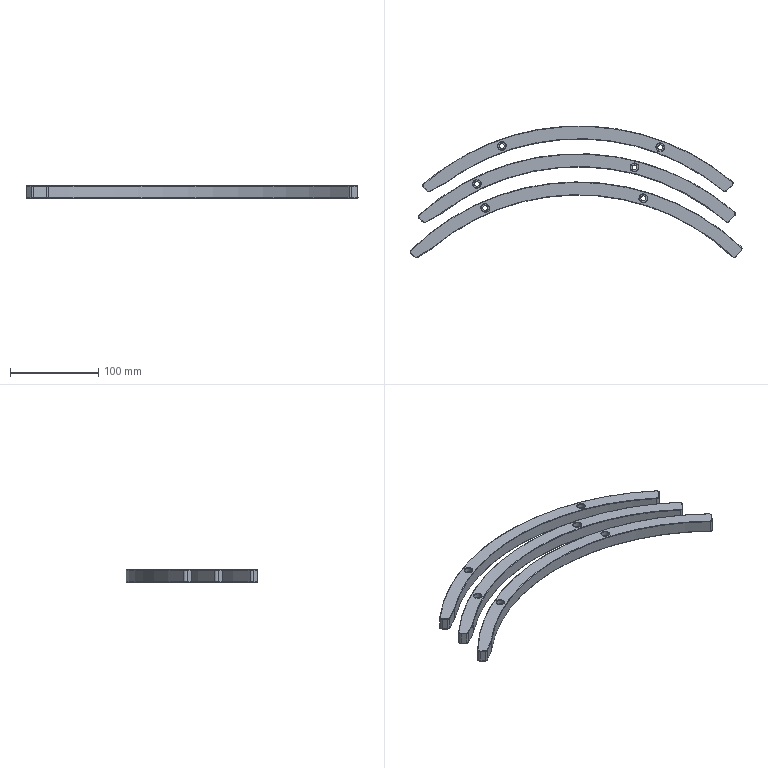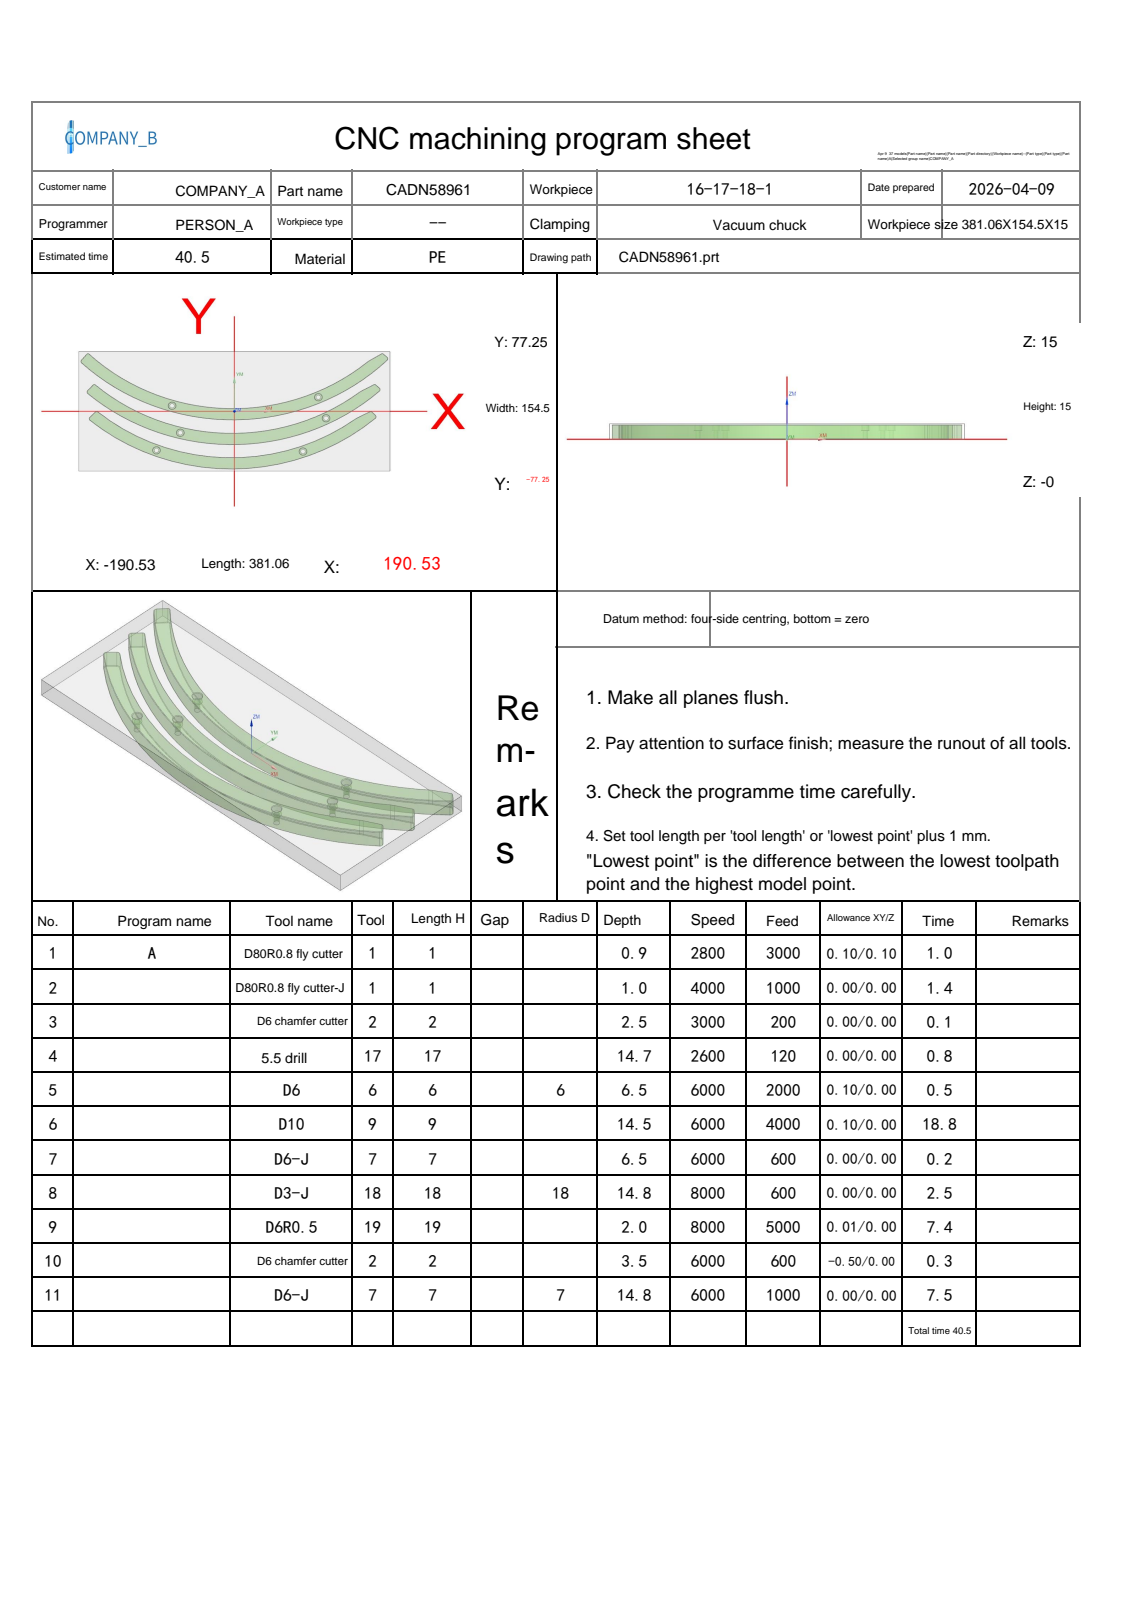NC program | NX | posted by the shop | part box 376.065 x 149.521 x 14 mm
Lines 1636 to 2623 of 3929:
N8 T18 M06
(D3-J  D=3. R=0. H=18 ce=0.00 di=0.00)
(D.N=18 MAX_Z=34. MIN_Z=0.2 Time=2.45M)
G00 G90 G54 X104.019 Y18.212 M03 S8000
G43 H18 Z34.
M08
Z9.
G01 Y18.335 Z8.994 F600.
X103.963 Y18.606 Z8.979
X103.847 Y18.857 Z8.965
X103.679 Y19.075 Z8.95
X103.465 Y19.25 Z8.936
X103.218 Y19.373 Z8.921
X102.949 Y19.437 Z8.907
X102.693 Y19.44 Z8.893
X102.417 Y19.383 Z8.879
X102.162 Y19.263 Z8.864
X101.941 Y19.088 Z8.849
X101.766 Y18.867 Z8.834
X101.646 Y18.612 Z8.819
X101.588 Y18.336 Z8.805
Y18.115 Z8.793
X101.646 Y17.839 Z8.778
X101.766 Y17.584 Z8.764
X101.941 Y17.363 Z8.749
X102.162 Y17.188 Z8.734
X102.417 Y17.068 Z8.719
X102.693 Y17.01 Z8.704
X102.914 Z8.693
X103.19 Y17.068 Z8.678
X103.445 Y17.187 Z8.663
X103.666 Y17.362 Z8.648
X103.841 Y17.583 Z8.634
X103.961 Y17.839 Z8.619
X104.019 Y18.115 Z8.604
Y18.335 Z8.593
X103.963 Y18.606 Z8.578
X103.847 Y18.857 Z8.564
X103.679 Y19.075 Z8.549
X103.465 Y19.25 Z8.535
X103.218 Y19.373 Z8.52
X102.949 Y19.437 Z8.506
X102.839 Y19.44 Z8.5
G41 D18
X102.804 Y19.475
G03 X101.553 Y18.225 Z8.426 I0.0 J-1.25
X102.803 Y16.975 Z8.352 I1.25 J0.0
X104.053 Y18.225 Z8.278 I0.0 J1.25
X102.804 Y19.475 Z8.204 I-1.25 J0.0
X101.553 Y18.225 Z8.129 I0.0 J-1.25
X102.803 Y16.975 Z8.055 I1.25 J0.0
X104.053 Y18.225 Z7.981 I0.0 J1.25
X102.804 Y19.475 Z7.907 I-1.25 J0.0
X101.553 Y18.225 Z7.833 I0.0 J-1.25
X102.803 Y16.975 Z7.759 I1.25 J0.0
X104.053 Y18.225 Z7.685 I0.0 J1.25
X102.804 Y19.475 Z7.611 I-1.25 J0.0
X101.553 Y18.225 Z7.537 I0.0 J-1.25
X102.803 Y16.975 Z7.463 I1.25 J0.0
X104.053 Y18.225 Z7.388 I0.0 J1.25
X102.804 Y19.475 Z7.314 I-1.25 J0.0
X101.553 Y18.225 Z7.24 I0.0 J-1.25
X102.803 Y16.975 Z7.166 I1.25 J0.0
X104.053 Y18.225 Z7.092 I0.0 J1.25
X102.804 Y19.475 Z7.018 I-1.25 J0.0
X101.553 Y18.225 Z6.944 I0.0 J-1.25
X102.803 Y16.975 Z6.87 I1.25 J0.0
X104.053 Y18.225 Z6.796 I0.0 J1.25
X102.804 Y19.475 Z6.721 I-1.25 J0.0
X101.553 Y18.225 Z6.647 I0.0 J-1.25
X102.803 Y16.975 Z6.573 I1.25 J0.0
X104.053 Y18.225 Z6.499 I0.0 J1.25
X102.804 Y19.475 Z6.425 I-1.25 J0.0
X101.553 Y18.225 Z6.351 I0.0 J-1.25
X102.803 Y16.975 Z6.277 I1.25 J0.0
X104.053 Y18.225 Z6.203 I0.0 J1.25
X102.804 Y19.475 Z6.129 I-1.25 J0.0
X101.553 Y18.225 Z6.054 I0.0 J-1.25
X102.803 Y16.975 Z5.98 I1.25 J0.0
X104.053 Y18.225 Z5.906 I0.0 J1.25
X102.804 Y19.475 Z5.832 I-1.25 J0.0
X101.553 Y18.225 Z5.758 I0.0 J-1.25
X102.803 Y16.975 Z5.684 I1.25 J0.0
X104.053 Y18.225 Z5.61 I0.0 J1.25
X102.804 Y19.475 Z5.536 I-1.25 J0.0
X101.553 Y18.225 Z5.462 I0.0 J-1.25
X102.803 Y16.975 Z5.388 I1.25 J0.0
X104.053 Y18.225 Z5.313 I0.0 J1.25
X102.804 Y19.475 Z5.239 I-1.25 J0.0
X101.553 Y18.225 Z5.165 I0.0 J-1.25
X102.803 Y16.975 Z5.091 I1.25 J0.0
X104.053 Y18.225 Z5.017 I0.0 J1.25
X102.804 Y19.475 Z4.943 I-1.25 J0.0
X101.553 Y18.225 Z4.869 I0.0 J-1.25
X102.803 Y16.975 Z4.795 I1.25 J0.0
X104.053 Y18.225 Z4.721 I0.0 J1.25
X102.804 Y19.475 Z4.646 I-1.25 J0.0
X101.553 Y18.225 Z4.572 I0.0 J-1.25
X102.803 Y16.975 Z4.498 I1.25 J0.0
X104.053 Y18.225 Z4.424 I0.0 J1.25
X102.804 Y19.475 Z4.35 I-1.25 J0.0
X101.553 Y18.225 Z4.276 I0.0 J-1.25
X102.803 Y16.975 Z4.202 I1.25 J0.0
X104.053 Y18.225 Z4.128 I0.0 J1.25
X102.804 Y19.475 Z4.054 I-1.25 J0.0
X101.553 Y18.225 Z3.979 I0.0 J-1.25
X102.803 Y16.975 Z3.905 I1.25 J0.0
X104.053 Y18.225 Z3.831 I0.0 J1.25
X102.804 Y19.475 Z3.757 I-1.25 J0.0
X101.553 Y18.225 Z3.683 I0.0 J-1.25
X102.803 Y16.975 Z3.609 I1.25 J0.0
X104.053 Y18.225 Z3.535 I0.0 J1.25
X102.804 Y19.475 Z3.461 I-1.25 J0.0
X101.553 Y18.225 Z3.387 I0.0 J-1.25
X102.803 Y16.975 Z3.313 I1.25 J0.0
X104.053 Y18.225 Z3.238 I0.0 J1.25
X102.804 Y19.475 Z3.164 I-1.25 J0.0
X101.553 Y18.225 Z3.09 I0.0 J-1.25
X102.803 Y16.975 Z3.016 I1.25 J0.0
X104.053 Y18.225 Z2.942 I0.0 J1.25
X102.804 Y19.475 Z2.868 I-1.25 J0.0
X101.553 Y18.225 Z2.794 I0.0 J-1.25
X102.803 Y16.975 Z2.72 I1.25 J0.0
X104.053 Y18.225 Z2.646 I0.0 J1.25
X102.804 Y19.475 Z2.571 I-1.25 J0.0
X101.553 Y18.225 Z2.497 I0.0 J-1.25
X102.803 Y16.975 Z2.423 I1.25 J0.0
X104.053 Y18.225 Z2.349 I0.0 J1.25
X102.804 Y19.475 Z2.275 I-1.25 J0.0
X101.553 Y18.225 Z2.201 I0.0 J-1.25
X102.803 Y16.975 Z2.127 I1.25 J0.0
X104.053 Y18.225 Z2.053 I0.0 J1.25
X102.804 Y19.475 Z1.979 I-1.25 J0.0
X101.553 Y18.225 Z1.904 I0.0 J-1.25
X102.803 Y16.975 Z1.83 I1.25 J0.0
X104.053 Y18.225 Z1.756 I0.0 J1.25
X102.804 Y19.475 Z1.682 I-1.25 J0.0
X101.553 Y18.225 Z1.608 I0.0 J-1.25
X102.803 Y16.975 Z1.534 I1.25 J0.0
X104.053 Y18.225 Z1.46 I0.0 J1.25
X102.804 Y19.475 Z1.386 I-1.25 J0.0
X101.553 Y18.225 Z1.312 I0.0 J-1.25
X102.803 Y16.975 Z1.238 I1.25 J0.0
X104.053 Y18.225 Z1.163 I0.0 J1.25
X102.804 Y19.475 Z1.089 I-1.25 J0.0
X101.553 Y18.225 Z1.015 I0.0 J-1.25
X102.803 Y16.975 Z.941 I1.25 J0.0
X104.053 Y18.225 Z.867 I0.0 J1.25
X102.804 Y19.475 Z.793 I-1.25 J0.0
X101.553 Y18.225 Z.719 I0.0 J-1.25
X102.803 Y16.975 Z.645 I1.25 J0.0
X104.053 Y18.225 Z.571 I0.0 J1.25
X102.804 Y19.475 Z.496 I-1.25 J0.0
X101.553 Y18.225 Z.422 I0.0 J-1.25
X102.803 Y16.975 Z.348 I1.25 J0.0
X104.053 Y18.225 Z.274 I0.0 J1.25
X102.804 Y19.475 Z.2 I-1.25 J0.0
X101.553 Y18.225 I0.0 J-1.25
X102.803 Y16.975 I1.25 J0.0
X104.053 Y18.225 I0.0 J1.25
X102.804 Y19.475 I-1.25 J0.0
X102.41 Y19.412 I0.0 J-1.25
G01 X102.385 Y19.401
X102.372 Y19.376
X102.379 Y19.349
G40 X102.394 Y19.301
Z1.2
G00 Z34.
X110.977 Y-8.948
Z9.
G01 Y-9.071 Z8.994
X111.033 Y-9.342 Z8.979
X111.148 Y-9.593 Z8.965
X111.317 Y-9.811 Z8.95
X111.531 Y-9.986 Z8.936
X111.778 Y-10.109 Z8.921
X112.047 Y-10.173 Z8.907
X112.303 Y-10.176 Z8.893
X112.579 Y-10.119 Z8.879
X112.834 Y-9.999 Z8.864
X113.055 Y-9.824 Z8.849
X113.23 Y-9.603 Z8.834
X113.35 Y-9.348 Z8.819
X113.408 Y-9.072 Z8.805
Y-8.851 Z8.793
X113.35 Y-8.575 Z8.778
X113.23 Y-8.32 Z8.764
X113.055 Y-8.098 Z8.749
X112.834 Y-7.923 Z8.734
X112.579 Y-7.804 Z8.719
X112.303 Y-7.746 Z8.704
X112.082 Z8.693
X111.806 Y-7.804 Z8.678
X111.551 Y-7.923 Z8.663
X111.33 Y-8.098 Z8.648
X111.155 Y-8.319 Z8.634
X111.035 Y-8.575 Z8.619
X110.977 Y-8.851 Z8.604
Y-9.071 Z8.593
X111.033 Y-9.342 Z8.578
X111.148 Y-9.593 Z8.564
X111.317 Y-9.811 Z8.549
X111.531 Y-9.986 Z8.535
X111.778 Y-10.109 Z8.52
X112.047 Y-10.173 Z8.506
X112.157 Y-10.176 Z8.5
G41 D18
X112.192 Y-10.211
G03 X113.442 Y-8.961 Z8.426 I0.0 J1.25
X112.192 Y-7.711 Z8.352 I-1.25 J0.0
X110.942 Y-8.961 Z8.278 I0.0 J-1.25
X112.192 Y-10.211 Z8.204 I1.25 J0.0
X113.442 Y-8.961 Z8.129 I0.0 J1.25
X112.192 Y-7.711 Z8.055 I-1.25 J0.0
X110.942 Y-8.961 Z7.981 I0.0 J-1.25
X112.192 Y-10.211 Z7.907 I1.25 J0.0
X113.442 Y-8.961 Z7.833 I0.0 J1.25
X112.192 Y-7.711 Z7.759 I-1.25 J0.0
X110.942 Y-8.961 Z7.685 I0.0 J-1.25
X112.192 Y-10.211 Z7.611 I1.25 J0.0
X113.442 Y-8.961 Z7.537 I0.0 J1.25
X112.192 Y-7.711 Z7.463 I-1.25 J0.0
X110.942 Y-8.961 Z7.388 I0.0 J-1.25
X112.192 Y-10.211 Z7.314 I1.25 J0.0
X113.442 Y-8.961 Z7.24 I0.0 J1.25
X112.192 Y-7.711 Z7.166 I-1.25 J0.0
X110.942 Y-8.961 Z7.092 I0.0 J-1.25
X112.192 Y-10.211 Z7.018 I1.25 J0.0
X113.442 Y-8.961 Z6.944 I0.0 J1.25
X112.192 Y-7.711 Z6.87 I-1.25 J0.0
X110.942 Y-8.961 Z6.796 I0.0 J-1.25
X112.192 Y-10.211 Z6.721 I1.25 J0.0
X113.442 Y-8.961 Z6.647 I0.0 J1.25
X112.192 Y-7.711 Z6.573 I-1.25 J0.0
X110.942 Y-8.961 Z6.499 I0.0 J-1.25
X112.192 Y-10.211 Z6.425 I1.25 J0.0
X113.442 Y-8.961 Z6.351 I0.0 J1.25
X112.192 Y-7.711 Z6.277 I-1.25 J0.0
X110.942 Y-8.961 Z6.203 I0.0 J-1.25
X112.192 Y-10.211 Z6.129 I1.25 J0.0
X113.442 Y-8.961 Z6.054 I0.0 J1.25
X112.192 Y-7.711 Z5.98 I-1.25 J0.0
X110.942 Y-8.961 Z5.906 I0.0 J-1.25
X112.192 Y-10.211 Z5.832 I1.25 J0.0
X113.442 Y-8.961 Z5.758 I0.0 J1.25
X112.192 Y-7.711 Z5.684 I-1.25 J0.0
X110.942 Y-8.961 Z5.61 I0.0 J-1.25
X112.192 Y-10.211 Z5.536 I1.25 J0.0
X113.442 Y-8.961 Z5.462 I0.0 J1.25
X112.192 Y-7.711 Z5.388 I-1.25 J0.0
X110.942 Y-8.961 Z5.313 I0.0 J-1.25
X112.192 Y-10.211 Z5.239 I1.25 J0.0
X113.442 Y-8.961 Z5.165 I0.0 J1.25
X112.192 Y-7.711 Z5.091 I-1.25 J0.0
X110.942 Y-8.961 Z5.017 I0.0 J-1.25
X112.192 Y-10.211 Z4.943 I1.25 J0.0
X113.442 Y-8.961 Z4.869 I0.0 J1.25
X112.192 Y-7.711 Z4.795 I-1.25 J0.0
X110.942 Y-8.961 Z4.721 I0.0 J-1.25
X112.192 Y-10.211 Z4.646 I1.25 J0.0
X113.442 Y-8.961 Z4.572 I0.0 J1.25
X112.192 Y-7.711 Z4.498 I-1.25 J0.0
X110.942 Y-8.961 Z4.424 I0.0 J-1.25
X112.192 Y-10.211 Z4.35 I1.25 J0.0
X113.442 Y-8.961 Z4.276 I0.0 J1.25
X112.192 Y-7.711 Z4.202 I-1.25 J0.0
X110.942 Y-8.961 Z4.128 I0.0 J-1.25
X112.192 Y-10.211 Z4.054 I1.25 J0.0
X113.442 Y-8.961 Z3.979 I0.0 J1.25
X112.192 Y-7.711 Z3.905 I-1.25 J0.0
X110.942 Y-8.961 Z3.831 I0.0 J-1.25
X112.192 Y-10.211 Z3.757 I1.25 J0.0
X113.442 Y-8.961 Z3.683 I0.0 J1.25
X112.192 Y-7.711 Z3.609 I-1.25 J0.0
X110.942 Y-8.961 Z3.535 I0.0 J-1.25
X112.192 Y-10.211 Z3.461 I1.25 J0.0
X113.442 Y-8.961 Z3.387 I0.0 J1.25
X112.192 Y-7.711 Z3.313 I-1.25 J0.0
X110.942 Y-8.961 Z3.238 I0.0 J-1.25
X112.192 Y-10.211 Z3.164 I1.25 J0.0
X113.442 Y-8.961 Z3.09 I0.0 J1.25
X112.192 Y-7.711 Z3.016 I-1.25 J0.0
X110.942 Y-8.961 Z2.942 I0.0 J-1.25
X112.192 Y-10.211 Z2.868 I1.25 J0.0
X113.442 Y-8.961 Z2.794 I0.0 J1.25
X112.192 Y-7.711 Z2.72 I-1.25 J0.0
X110.942 Y-8.961 Z2.646 I0.0 J-1.25
X112.192 Y-10.211 Z2.571 I1.25 J0.0
X113.442 Y-8.961 Z2.497 I0.0 J1.25
X112.192 Y-7.711 Z2.423 I-1.25 J0.0
X110.942 Y-8.961 Z2.349 I0.0 J-1.25
X112.192 Y-10.211 Z2.275 I1.25 J0.0
X113.442 Y-8.961 Z2.201 I0.0 J1.25
X112.192 Y-7.711 Z2.127 I-1.25 J0.0
X110.942 Y-8.961 Z2.053 I0.0 J-1.25
X112.192 Y-10.211 Z1.979 I1.25 J0.0
X113.442 Y-8.961 Z1.904 I0.0 J1.25
X112.192 Y-7.711 Z1.83 I-1.25 J0.0
X110.942 Y-8.961 Z1.756 I0.0 J-1.25
X112.192 Y-10.211 Z1.682 I1.25 J0.0
X113.442 Y-8.961 Z1.608 I0.0 J1.25
X112.192 Y-7.711 Z1.534 I-1.25 J0.0
X110.942 Y-8.961 Z1.46 I0.0 J-1.25
X112.192 Y-10.211 Z1.386 I1.25 J0.0
X113.442 Y-8.961 Z1.312 I0.0 J1.25
X112.192 Y-7.711 Z1.238 I-1.25 J0.0
X110.942 Y-8.961 Z1.163 I0.0 J-1.25
X112.192 Y-10.211 Z1.089 I1.25 J0.0
X113.442 Y-8.961 Z1.015 I0.0 J1.25
X112.192 Y-7.711 Z.941 I-1.25 J0.0
X110.942 Y-8.961 Z.867 I0.0 J-1.25
X112.192 Y-10.211 Z.793 I1.25 J0.0
X113.442 Y-8.961 Z.719 I0.0 J1.25
X112.192 Y-7.711 Z.645 I-1.25 J0.0
X110.942 Y-8.961 Z.571 I0.0 J-1.25
X112.192 Y-10.211 Z.496 I1.25 J0.0
X113.442 Y-8.961 Z.422 I0.0 J1.25
X112.192 Y-7.711 Z.348 I-1.25 J0.0
X110.942 Y-8.961 Z.274 I0.0 J-1.25
X112.192 Y-10.211 Z.2 I1.25 J0.0
X113.442 Y-8.961 I0.0 J1.25
X112.192 Y-7.711 I-1.25 J0.0
X110.942 Y-8.961 I0.0 J-1.25
X112.192 Y-10.211 I1.25 J0.0
X112.585 Y-10.148 I0.0 J1.25
G01 X112.611 Y-10.137
X112.624 Y-10.111
X112.617 Y-10.085
G40 X112.601 Y-10.037
Z1.2
G00 Z34.
X82.776 Y-51.923
Z9.
G01 Y-52.046 Z8.994
X82.832 Y-52.317 Z8.979
X82.947 Y-52.567 Z8.965
X83.116 Y-52.786 Z8.95
X83.33 Y-52.961 Z8.936
X83.577 Y-53.084 Z8.921
X83.846 Y-53.147 Z8.907
X84.102 Y-53.151 Z8.893
X84.378 Y-53.093 Z8.879
X84.633 Y-52.974 Z8.864
X84.854 Y-52.799 Z8.849
X85.029 Y-52.578 Z8.834
X85.149 Y-52.322 Z8.819
X85.207 Y-52.046 Z8.805
Y-51.826 Z8.793
X85.149 Y-51.55 Z8.778
X85.029 Y-51.294 Z8.764
X84.854 Y-51.073 Z8.749
X84.633 Y-50.898 Z8.734
X84.378 Y-50.779 Z8.719
X84.102 Y-50.721 Z8.704
X83.881 Z8.693
X83.605 Y-50.779 Z8.678
X83.35 Y-50.898 Z8.663
X83.129 Y-51.073 Z8.648
X82.954 Y-51.294 Z8.634
X82.834 Y-51.55 Z8.619
X82.776 Y-51.826 Z8.604
Y-52.046 Z8.593
X82.832 Y-52.317 Z8.578
X82.947 Y-52.567 Z8.564
X83.116 Y-52.786 Z8.549
X83.33 Y-52.961 Z8.535
X83.577 Y-53.084 Z8.52
X83.846 Y-53.147 Z8.506
X83.956 Y-53.151 Z8.5
G41 D18
X83.991 Y-53.186
G03 X85.242 Y-51.936 Z8.426 I0.0 J1.25
X83.992 Y-50.686 Z8.352 I-1.25 J0.0
X82.742 Y-51.936 Z8.278 I0.0 J-1.25
X83.991 Y-53.186 Z8.204 I1.25 J0.0
X85.242 Y-51.936 Z8.129 I0.0 J1.25
X83.992 Y-50.686 Z8.055 I-1.25 J0.0
X82.742 Y-51.936 Z7.981 I0.0 J-1.25
X83.991 Y-53.186 Z7.907 I1.25 J0.0
X85.242 Y-51.936 Z7.833 I0.0 J1.25
X83.992 Y-50.686 Z7.759 I-1.25 J0.0
X82.742 Y-51.936 Z7.685 I0.0 J-1.25
X83.991 Y-53.186 Z7.611 I1.25 J0.0
X85.242 Y-51.936 Z7.537 I0.0 J1.25
X83.992 Y-50.686 Z7.463 I-1.25 J0.0
X82.742 Y-51.936 Z7.388 I0.0 J-1.25
X83.991 Y-53.186 Z7.314 I1.25 J0.0
X85.242 Y-51.936 Z7.24 I0.0 J1.25
X83.992 Y-50.686 Z7.166 I-1.25 J0.0
X82.742 Y-51.936 Z7.092 I0.0 J-1.25
X83.991 Y-53.186 Z7.018 I1.25 J0.0
X85.242 Y-51.936 Z6.944 I0.0 J1.25
X83.992 Y-50.686 Z6.87 I-1.25 J0.0
X82.742 Y-51.936 Z6.796 I0.0 J-1.25
X83.991 Y-53.186 Z6.721 I1.25 J0.0
X85.242 Y-51.936 Z6.647 I0.0 J1.25
X83.992 Y-50.686 Z6.573 I-1.25 J0.0
X82.742 Y-51.936 Z6.499 I0.0 J-1.25
X83.991 Y-53.186 Z6.425 I1.25 J0.0
X85.242 Y-51.936 Z6.351 I0.0 J1.25
X83.992 Y-50.686 Z6.277 I-1.25 J0.0
X82.742 Y-51.936 Z6.203 I0.0 J-1.25
X83.991 Y-53.186 Z6.129 I1.25 J0.0
X85.242 Y-51.936 Z6.054 I0.0 J1.25
X83.992 Y-50.686 Z5.98 I-1.25 J0.0
X82.742 Y-51.936 Z5.906 I0.0 J-1.25
X83.991 Y-53.186 Z5.832 I1.25 J0.0
X85.242 Y-51.936 Z5.758 I0.0 J1.25
X83.992 Y-50.686 Z5.684 I-1.25 J0.0
X82.742 Y-51.936 Z5.61 I0.0 J-1.25
X83.991 Y-53.186 Z5.536 I1.25 J0.0
X85.242 Y-51.936 Z5.462 I0.0 J1.25
X83.992 Y-50.686 Z5.388 I-1.25 J0.0
X82.742 Y-51.936 Z5.313 I0.0 J-1.25
X83.991 Y-53.186 Z5.239 I1.25 J0.0
X85.242 Y-51.936 Z5.165 I0.0 J1.25
X83.992 Y-50.686 Z5.091 I-1.25 J0.0
X82.742 Y-51.936 Z5.017 I0.0 J-1.25
X83.991 Y-53.186 Z4.943 I1.25 J0.0
X85.242 Y-51.936 Z4.869 I0.0 J1.25
X83.992 Y-50.686 Z4.795 I-1.25 J0.0
X82.742 Y-51.936 Z4.721 I0.0 J-1.25
X83.991 Y-53.186 Z4.646 I1.25 J0.0
X85.242 Y-51.936 Z4.572 I0.0 J1.25
X83.992 Y-50.686 Z4.498 I-1.25 J0.0
X82.742 Y-51.936 Z4.424 I0.0 J-1.25
X83.991 Y-53.186 Z4.35 I1.25 J0.0
X85.242 Y-51.936 Z4.276 I0.0 J1.25
X83.992 Y-50.686 Z4.202 I-1.25 J0.0
X82.742 Y-51.936 Z4.128 I0.0 J-1.25
X83.991 Y-53.186 Z4.054 I1.25 J0.0
X85.242 Y-51.936 Z3.979 I0.0 J1.25
X83.992 Y-50.686 Z3.905 I-1.25 J0.0
X82.742 Y-51.936 Z3.831 I0.0 J-1.25
X83.991 Y-53.186 Z3.757 I1.25 J0.0
X85.242 Y-51.936 Z3.683 I0.0 J1.25
X83.992 Y-50.686 Z3.609 I-1.25 J0.0
X82.742 Y-51.936 Z3.535 I0.0 J-1.25
X83.991 Y-53.186 Z3.461 I1.25 J0.0
X85.242 Y-51.936 Z3.387 I0.0 J1.25
X83.992 Y-50.686 Z3.313 I-1.25 J0.0
X82.742 Y-51.936 Z3.238 I0.0 J-1.25
X83.991 Y-53.186 Z3.164 I1.25 J0.0
X85.242 Y-51.936 Z3.09 I0.0 J1.25
X83.992 Y-50.686 Z3.016 I-1.25 J0.0
X82.742 Y-51.936 Z2.942 I0.0 J-1.25
X83.991 Y-53.186 Z2.868 I1.25 J0.0
X85.242 Y-51.936 Z2.794 I0.0 J1.25
X83.992 Y-50.686 Z2.72 I-1.25 J0.0
X82.742 Y-51.936 Z2.646 I0.0 J-1.25
X83.991 Y-53.186 Z2.571 I1.25 J0.0
X85.242 Y-51.936 Z2.497 I0.0 J1.25
X83.992 Y-50.686 Z2.423 I-1.25 J0.0
X82.742 Y-51.936 Z2.349 I0.0 J-1.25
X83.991 Y-53.186 Z2.275 I1.25 J0.0
X85.242 Y-51.936 Z2.201 I0.0 J1.25
X83.992 Y-50.686 Z2.127 I-1.25 J0.0
X82.742 Y-51.936 Z2.053 I0.0 J-1.25
X83.991 Y-53.186 Z1.979 I1.25 J0.0
X85.242 Y-51.936 Z1.904 I0.0 J1.25
X83.992 Y-50.686 Z1.83 I-1.25 J0.0
X82.742 Y-51.936 Z1.756 I0.0 J-1.25
X83.991 Y-53.186 Z1.682 I1.25 J0.0
X85.242 Y-51.936 Z1.608 I0.0 J1.25
X83.992 Y-50.686 Z1.534 I-1.25 J0.0
X82.742 Y-51.936 Z1.46 I0.0 J-1.25
X83.991 Y-53.186 Z1.386 I1.25 J0.0
X85.242 Y-51.936 Z1.312 I0.0 J1.25
X83.992 Y-50.686 Z1.238 I-1.25 J0.0
X82.742 Y-51.936 Z1.163 I0.0 J-1.25
X83.991 Y-53.186 Z1.089 I1.25 J0.0
X85.242 Y-51.936 Z1.015 I0.0 J1.25
X83.992 Y-50.686 Z.941 I-1.25 J0.0
X82.742 Y-51.936 Z.867 I0.0 J-1.25
X83.991 Y-53.186 Z.793 I1.25 J0.0
X85.242 Y-51.936 Z.719 I0.0 J1.25
X83.992 Y-50.686 Z.645 I-1.25 J0.0
X82.742 Y-51.936 Z.571 I0.0 J-1.25
X83.991 Y-53.186 Z.496 I1.25 J0.0
X85.242 Y-51.936 Z.422 I0.0 J1.25
X83.992 Y-50.686 Z.348 I-1.25 J0.0
X82.742 Y-51.936 Z.274 I0.0 J-1.25
X83.991 Y-53.186 Z.2 I1.25 J0.0
X85.242 Y-51.936 I0.0 J1.25
X83.992 Y-50.686 I-1.25 J0.0
X82.742 Y-51.936 I0.0 J-1.25
X83.991 Y-53.186 I1.25 J0.0
X84.385 Y-53.123 I0.0 J1.25
G01 X84.41 Y-53.112
X84.423 Y-53.086
X84.416 Y-53.059
G40 X84.401 Y-53.012
Z1.2
G00 Z34.
X-75.04 Y7.218
Z9.
G01 Y7.342 Z8.994
X-75.096 Y7.612 Z8.979
X-75.212 Y7.863 Z8.965
X-75.38 Y8.082 Z8.95
X-75.594 Y8.257 Z8.936
X-75.841 Y8.379 Z8.921
X-76.11 Y8.443 Z8.907
X-76.366 Y8.447 Z8.893
X-76.642 Y8.389 Z8.879
X-76.897 Y8.27 Z8.864
X-77.118 Y8.095 Z8.849
X-77.293 Y7.873 Z8.834
X-77.413 Y7.618 Z8.819
X-77.471 Y7.342 Z8.805
Y7.121 Z8.793
X-77.413 Y6.845 Z8.778
X-77.293 Y6.59 Z8.764
X-77.118 Y6.369 Z8.749
X-76.897 Y6.194 Z8.734
X-76.642 Y6.074 Z8.719
X-76.366 Y6.017 Z8.704
X-76.145 Z8.693
X-75.869 Y6.074 Z8.678
X-75.614 Y6.194 Z8.663
X-75.393 Y6.369 Z8.648
X-75.218 Y6.59 Z8.634
X-75.098 Y6.845 Z8.619
X-75.04 Y7.121 Z8.604
Y7.342 Z8.593
X-75.096 Y7.612 Z8.578
X-75.212 Y7.863 Z8.564
X-75.38 Y8.082 Z8.549
X-75.594 Y8.257 Z8.535
X-75.841 Y8.379 Z8.52
X-76.11 Y8.443 Z8.506
X-76.22 Y8.446 Z8.5
G41 D18
X-76.255 Y8.482
G03 X-77.506 Y7.232 Z8.426 I0.0 J-1.25
X-76.256 Y5.982 Z8.352 I1.25 J0.0
X-75.006 Y7.232 Z8.278 I0.0 J1.25
X-76.255 Y8.482 Z8.204 I-1.25 J0.0
X-77.506 Y7.232 Z8.129 I0.0 J-1.25
X-76.256 Y5.982 Z8.055 I1.25 J0.0
X-75.006 Y7.232 Z7.981 I0.0 J1.25
X-76.255 Y8.482 Z7.907 I-1.25 J0.0
X-77.506 Y7.232 Z7.833 I0.0 J-1.25
X-76.256 Y5.982 Z7.759 I1.25 J0.0
X-75.006 Y7.232 Z7.685 I0.0 J1.25
X-76.255 Y8.482 Z7.611 I-1.25 J0.0
X-77.506 Y7.232 Z7.537 I0.0 J-1.25
X-76.256 Y5.982 Z7.463 I1.25 J0.0
X-75.006 Y7.232 Z7.388 I0.0 J1.25
X-76.255 Y8.482 Z7.314 I-1.25 J0.0
X-77.506 Y7.232 Z7.24 I0.0 J-1.25
X-76.256 Y5.982 Z7.166 I1.25 J0.0
X-75.006 Y7.232 Z7.092 I0.0 J1.25
X-76.255 Y8.482 Z7.018 I-1.25 J0.0
X-77.506 Y7.232 Z6.944 I0.0 J-1.25
X-76.256 Y5.982 Z6.87 I1.25 J0.0
X-75.006 Y7.232 Z6.796 I0.0 J1.25
X-76.255 Y8.482 Z6.721 I-1.25 J0.0
X-77.506 Y7.232 Z6.647 I0.0 J-1.25
X-76.256 Y5.982 Z6.573 I1.25 J0.0
X-75.006 Y7.232 Z6.499 I0.0 J1.25
X-76.255 Y8.482 Z6.425 I-1.25 J0.0
X-77.506 Y7.232 Z6.351 I0.0 J-1.25
X-76.256 Y5.982 Z6.277 I1.25 J0.0
X-75.006 Y7.232 Z6.203 I0.0 J1.25
X-76.255 Y8.482 Z6.129 I-1.25 J0.0
X-77.506 Y7.232 Z6.054 I0.0 J-1.25
X-76.256 Y5.982 Z5.98 I1.25 J0.0
X-75.006 Y7.232 Z5.906 I0.0 J1.25
X-76.255 Y8.482 Z5.832 I-1.25 J0.0
X-77.506 Y7.232 Z5.758 I0.0 J-1.25
X-76.256 Y5.982 Z5.684 I1.25 J0.0
X-75.006 Y7.232 Z5.61 I0.0 J1.25
X-76.255 Y8.482 Z5.536 I-1.25 J0.0
X-77.506 Y7.232 Z5.462 I0.0 J-1.25
X-76.256 Y5.982 Z5.388 I1.25 J0.0
X-75.006 Y7.232 Z5.313 I0.0 J1.25
X-76.255 Y8.482 Z5.239 I-1.25 J0.0
X-77.506 Y7.232 Z5.165 I0.0 J-1.25
X-76.256 Y5.982 Z5.091 I1.25 J0.0
X-75.006 Y7.232 Z5.017 I0.0 J1.25
X-76.255 Y8.482 Z4.943 I-1.25 J0.0
X-77.506 Y7.232 Z4.869 I0.0 J-1.25
X-76.256 Y5.982 Z4.795 I1.25 J0.0
X-75.006 Y7.232 Z4.721 I0.0 J1.25
X-76.255 Y8.482 Z4.646 I-1.25 J0.0
X-77.506 Y7.232 Z4.572 I0.0 J-1.25
X-76.256 Y5.982 Z4.498 I1.25 J0.0
X-75.006 Y7.232 Z4.424 I0.0 J1.25
X-76.255 Y8.482 Z4.35 I-1.25 J0.0
X-77.506 Y7.232 Z4.276 I0.0 J-1.25
X-76.256 Y5.982 Z4.202 I1.25 J0.0
X-75.006 Y7.232 Z4.128 I0.0 J1.25
X-76.255 Y8.482 Z4.054 I-1.25 J0.0
X-77.506 Y7.232 Z3.979 I0.0 J-1.25
X-76.256 Y5.982 Z3.905 I1.25 J0.0
X-75.006 Y7.232 Z3.831 I0.0 J1.25
X-76.255 Y8.482 Z3.757 I-1.25 J0.0
X-77.506 Y7.232 Z3.683 I0.0 J-1.25
X-76.256 Y5.982 Z3.609 I1.25 J0.0
X-75.006 Y7.232 Z3.535 I0.0 J1.25
X-76.255 Y8.482 Z3.461 I-1.25 J0.0
X-77.506 Y7.232 Z3.387 I0.0 J-1.25
X-76.256 Y5.982 Z3.313 I1.25 J0.0
X-75.006 Y7.232 Z3.238 I0.0 J1.25
X-76.255 Y8.482 Z3.164 I-1.25 J0.0
X-77.506 Y7.232 Z3.09 I0.0 J-1.25
X-76.256 Y5.982 Z3.016 I1.25 J0.0
X-75.006 Y7.232 Z2.942 I0.0 J1.25
X-76.255 Y8.482 Z2.868 I-1.25 J0.0
X-77.506 Y7.232 Z2.794 I0.0 J-1.25
X-76.256 Y5.982 Z2.72 I1.25 J0.0
X-75.006 Y7.232 Z2.646 I0.0 J1.25
X-76.255 Y8.482 Z2.571 I-1.25 J0.0
X-77.506 Y7.232 Z2.497 I0.0 J-1.25
X-76.256 Y5.982 Z2.423 I1.25 J0.0
X-75.006 Y7.232 Z2.349 I0.0 J1.25
X-76.255 Y8.482 Z2.275 I-1.25 J0.0
X-77.506 Y7.232 Z2.201 I0.0 J-1.25
X-76.256 Y5.982 Z2.127 I1.25 J0.0
X-75.006 Y7.232 Z2.053 I0.0 J1.25
X-76.255 Y8.482 Z1.979 I-1.25 J0.0
X-77.506 Y7.232 Z1.904 I0.0 J-1.25
X-76.256 Y5.982 Z1.83 I1.25 J0.0
X-75.006 Y7.232 Z1.756 I0.0 J1.25
X-76.255 Y8.482 Z1.682 I-1.25 J0.0
X-77.506 Y7.232 Z1.608 I0.0 J-1.25
X-76.256 Y5.982 Z1.534 I1.25 J0.0
X-75.006 Y7.232 Z1.46 I0.0 J1.25
X-76.255 Y8.482 Z1.386 I-1.25 J0.0
X-77.506 Y7.232 Z1.312 I0.0 J-1.25
X-76.256 Y5.982 Z1.238 I1.25 J0.0
X-75.006 Y7.232 Z1.163 I0.0 J1.25
X-76.255 Y8.482 Z1.089 I-1.25 J0.0
X-77.506 Y7.232 Z1.015 I0.0 J-1.25
X-76.256 Y5.982 Z.941 I1.25 J0.0
X-75.006 Y7.232 Z.867 I0.0 J1.25
X-76.255 Y8.482 Z.793 I-1.25 J0.0
X-77.506 Y7.232 Z.719 I0.0 J-1.25
X-76.256 Y5.982 Z.645 I1.25 J0.0
X-75.006 Y7.232 Z.571 I0.0 J1.25
X-76.255 Y8.482 Z.496 I-1.25 J0.0
X-77.506 Y7.232 Z.422 I0.0 J-1.25
X-76.256 Y5.982 Z.348 I1.25 J0.0
X-75.006 Y7.232 Z.274 I0.0 J1.25
X-76.255 Y8.482 Z.2 I-1.25 J0.0
X-77.506 Y7.232 I0.0 J-1.25
X-76.256 Y5.982 I1.25 J0.0
X-75.006 Y7.232 I0.0 J1.25
X-76.255 Y8.482 I-1.25 J0.0
X-76.649 Y8.418 I0.0 J-1.25
G01 X-76.674 Y8.407
X-76.687 Y8.382
X-76.68 Y8.355
G40 X-76.665 Y8.308
Z1.2
G00 Z34.
X-67.437 Y-27.69
Z9.
G01 Y-27.813 Z8.994
X-67.381 Y-28.084 Z8.979
X-67.266 Y-28.335 Z8.965
X-67.097 Y-28.553 Z8.95
X-66.884 Y-28.728 Z8.936
X-66.636 Y-28.851 Z8.921
X-66.368 Y-28.915 Z8.907
X-66.112 Y-28.918 Z8.893
X-65.836 Y-28.861 Z8.879
X-65.58 Y-28.741 Z8.864
X-65.359 Y-28.566 Z8.849
X-65.184 Y-28.345 Z8.834
X-65.065 Y-28.09 Z8.819
X-65.007 Y-27.814 Z8.805
Y-27.593 Z8.793
X-65.065 Y-27.317 Z8.778
X-65.184 Y-27.062 Z8.764
X-65.359 Y-26.84 Z8.749
X-65.58 Y-26.665 Z8.734
X-65.836 Y-26.546 Z8.719
X-66.112 Y-26.488 Z8.704
X-66.332 Z8.693
X-66.608 Y-26.546 Z8.678
X-66.864 Y-26.665 Z8.663
X-67.085 Y-26.84 Z8.648
X-67.26 Y-27.061 Z8.634
X-67.379 Y-27.317 Z8.619
X-67.437 Y-27.593 Z8.604
Y-27.813 Z8.593
X-67.381 Y-28.084 Z8.578
X-67.266 Y-28.335 Z8.564
X-67.097 Y-28.553 Z8.549
X-66.884 Y-28.728 Z8.535
X-66.636 Y-28.851 Z8.52
X-66.368 Y-28.915 Z8.506
X-66.258 Y-28.918 Z8.5
G41 D18
X-66.222 Y-28.953
G03 X-64.972 Y-27.703 Z8.426 I0.0 J1.25
X-66.222 Y-26.453 Z8.352 I-1.25 J0.0
X-67.472 Y-27.703 Z8.278 I0.0 J-1.25
X-66.222 Y-28.953 Z8.204 I1.25 J0.0
X-64.972 Y-27.703 Z8.129 I0.0 J1.25
X-66.222 Y-26.453 Z8.055 I-1.25 J0.0
X-67.472 Y-27.703 Z7.981 I0.0 J-1.25
X-66.222 Y-28.953 Z7.907 I1.25 J0.0
X-64.972 Y-27.703 Z7.833 I0.0 J1.25
X-66.222 Y-26.453 Z7.759 I-1.25 J0.0
X-67.472 Y-27.703 Z7.685 I0.0 J-1.25
X-66.222 Y-28.953 Z7.611 I1.25 J0.0
X-64.972 Y-27.703 Z7.537 I0.0 J1.25
X-66.222 Y-26.453 Z7.463 I-1.25 J0.0
X-67.472 Y-27.703 Z7.388 I0.0 J-1.25
X-66.222 Y-28.953 Z7.314 I1.25 J0.0
X-64.972 Y-27.703 Z7.24 I0.0 J1.25
X-66.222 Y-26.453 Z7.166 I-1.25 J0.0
X-67.472 Y-27.703 Z7.092 I0.0 J-1.25
X-66.222 Y-28.953 Z7.018 I1.25 J0.0
X-64.972 Y-27.703 Z6.944 I0.0 J1.25
X-66.222 Y-26.453 Z6.87 I-1.25 J0.0
X-67.472 Y-27.703 Z6.796 I0.0 J-1.25
X-66.222 Y-28.953 Z6.721 I1.25 J0.0
X-64.972 Y-27.703 Z6.647 I0.0 J1.25
X-66.222 Y-26.453 Z6.573 I-1.25 J0.0
X-67.472 Y-27.703 Z6.499 I0.0 J-1.25
X-66.222 Y-28.953 Z6.425 I1.25 J0.0
X-64.972 Y-27.703 Z6.351 I0.0 J1.25
X-66.222 Y-26.453 Z6.277 I-1.25 J0.0
X-67.472 Y-27.703 Z6.203 I0.0 J-1.25
X-66.222 Y-28.953 Z6.129 I1.25 J0.0
X-64.972 Y-27.703 Z6.054 I0.0 J1.25
X-66.222 Y-26.453 Z5.98 I-1.25 J0.0
X-67.472 Y-27.703 Z5.906 I0.0 J-1.25
X-66.222 Y-28.953 Z5.832 I1.25 J0.0
X-64.972 Y-27.703 Z5.758 I0.0 J1.25
X-66.222 Y-26.453 Z5.684 I-1.25 J0.0
X-67.472 Y-27.703 Z5.61 I0.0 J-1.25
X-66.222 Y-28.953 Z5.536 I1.25 J0.0
X-64.972 Y-27.703 Z5.462 I0.0 J1.25
X-66.222 Y-26.453 Z5.388 I-1.25 J0.0
X-67.472 Y-27.703 Z5.313 I0.0 J-1.25
X-66.222 Y-28.953 Z5.239 I1.25 J0.0
X-64.972 Y-27.703 Z5.165 I0.0 J1.25
X-66.222 Y-26.453 Z5.091 I-1.25 J0.0
X-67.472 Y-27.703 Z5.017 I0.0 J-1.25
X-66.222 Y-28.953 Z4.943 I1.25 J0.0
X-64.972 Y-27.703 Z4.869 I0.0 J1.25
X-66.222 Y-26.453 Z4.795 I-1.25 J0.0
X-67.472 Y-27.703 Z4.721 I0.0 J-1.25
X-66.222 Y-28.953 Z4.646 I1.25 J0.0
X-64.972 Y-27.703 Z4.572 I0.0 J1.25
X-66.222 Y-26.453 Z4.498 I-1.25 J0.0
X-67.472 Y-27.703 Z4.424 I0.0 J-1.25
X-66.222 Y-28.953 Z4.35 I1.25 J0.0
X-64.972 Y-27.703 Z4.276 I0.0 J1.25
X-66.222 Y-26.453 Z4.202 I-1.25 J0.0
X-67.472 Y-27.703 Z4.128 I0.0 J-1.25
X-66.222 Y-28.953 Z4.054 I1.25 J0.0
X-64.972 Y-27.703 Z3.979 I0.0 J1.25
X-66.222 Y-26.453 Z3.905 I-1.25 J0.0
X-67.472 Y-27.703 Z3.831 I0.0 J-1.25
X-66.222 Y-28.953 Z3.757 I1.25 J0.0
X-64.972 Y-27.703 Z3.683 I0.0 J1.25
X-66.222 Y-26.453 Z3.609 I-1.25 J0.0
X-67.472 Y-27.703 Z3.535 I0.0 J-1.25
X-66.222 Y-28.953 Z3.461 I1.25 J0.0
X-64.972 Y-27.703 Z3.387 I0.0 J1.25
X-66.222 Y-26.453 Z3.313 I-1.25 J0.0
X-67.472 Y-27.703 Z3.238 I0.0 J-1.25
X-66.222 Y-28.953 Z3.164 I1.25 J0.0
X-64.972 Y-27.703 Z3.09 I0.0 J1.25
X-66.222 Y-26.453 Z3.016 I-1.25 J0.0
X-67.472 Y-27.703 Z2.942 I0.0 J-1.25
X-66.222 Y-28.953 Z2.868 I1.25 J0.0
X-64.972 Y-27.703 Z2.794 I0.0 J1.25
X-66.222 Y-26.453 Z2.72 I-1.25 J0.0
X-67.472 Y-27.703 Z2.646 I0.0 J-1.25
X-66.222 Y-28.953 Z2.571 I1.25 J0.0
X-64.972 Y-27.703 Z2.497 I0.0 J1.25
X-66.222 Y-26.453 Z2.423 I-1.25 J0.0
X-67.472 Y-27.703 Z2.349 I0.0 J-1.25
X-66.222 Y-28.953 Z2.275 I1.25 J0.0
X-64.972 Y-27.703 Z2.201 I0.0 J1.25
X-66.222 Y-26.453 Z2.127 I-1.25 J0.0
X-67.472 Y-27.703 Z2.053 I0.0 J-1.25
X-66.222 Y-28.953 Z1.979 I1.25 J0.0
X-64.972 Y-27.703 Z1.904 I0.0 J1.25
X-66.222 Y-26.453 Z1.83 I-1.25 J0.0
X-67.472 Y-27.703 Z1.756 I0.0 J-1.25
X-66.222 Y-28.953 Z1.682 I1.25 J0.0
X-64.972 Y-27.703 Z1.608 I0.0 J1.25
X-66.222 Y-26.453 Z1.534 I-1.25 J0.0
X-67.472 Y-27.703 Z1.46 I0.0 J-1.25
X-66.222 Y-28.953 Z1.386 I1.25 J0.0
X-64.972 Y-27.703 Z1.312 I0.0 J1.25
X-66.222 Y-26.453 Z1.238 I-1.25 J0.0
X-67.472 Y-27.703 Z1.163 I0.0 J-1.25
X-66.222 Y-28.953 Z1.089 I1.25 J0.0
X-64.972 Y-27.703 Z1.015 I0.0 J1.25
X-66.222 Y-26.453 Z.941 I-1.25 J0.0
X-67.472 Y-27.703 Z.867 I0.0 J-1.25
X-66.222 Y-28.953 Z.793 I1.25 J0.0
X-64.972 Y-27.703 Z.719 I0.0 J1.25
X-66.222 Y-26.453 Z.645 I-1.25 J0.0
X-67.472 Y-27.703 Z.571 I0.0 J-1.25
X-66.222 Y-28.953 Z.496 I1.25 J0.0
X-64.972 Y-27.703 Z.422 I0.0 J1.25
X-66.222 Y-26.453 Z.348 I-1.25 J0.0
X-67.472 Y-27.703 Z.274 I0.0 J-1.25
X-66.222 Y-28.953 Z.2 I1.25 J0.0
X-64.972 Y-27.703 I0.0 J1.25
X-66.222 Y-26.453 I-1.25 J0.0
X-67.472 Y-27.703 I0.0 J-1.25
X-66.222 Y-28.953 I1.25 J0.0
X-65.829 Y-28.89 I0.0 J1.25
G01 X-65.804 Y-28.879
X-65.791 Y-28.853
X-65.797 Y-28.827
G40 X-65.813 Y-28.779
Z1.2
G00 Z34.
X-96.614 Y-50.424
Z9.
G01 Y-50.548 Z8.994
X-96.558 Y-50.818 Z8.979
X-96.442 Y-51.069 Z8.965
X-96.274 Y-51.288 Z8.95
X-96.06 Y-51.463 Z8.936
X-95.813 Y-51.585 Z8.921
X-95.544 Y-51.649 Z8.907
X-95.288 Y-51.653 Z8.893
X-95.012 Y-51.595 Z8.879
X-94.757 Y-51.475 Z8.864
X-94.536 Y-51.3 Z8.849
X-94.361 Y-51.079 Z8.834
X-94.241 Y-50.824 Z8.819
X-94.183 Y-50.548 Z8.805
Y-50.327 Z8.793
X-94.241 Y-50.051 Z8.778
X-94.361 Y-49.796 Z8.764
X-94.536 Y-49.575 Z8.749
X-94.757 Y-49.4 Z8.734
X-95.012 Y-49.28 Z8.719
X-95.288 Y-49.222 Z8.704
X-95.509 Z8.693
X-95.785 Y-49.28 Z8.678
X-96.04 Y-49.4 Z8.663
X-96.261 Y-49.575 Z8.648
X-96.436 Y-49.796 Z8.634
X-96.556 Y-50.051 Z8.619
X-96.614 Y-50.327 Z8.604
Y-50.548 Z8.593
X-96.558 Y-50.818 Z8.578
X-96.442 Y-51.069 Z8.564
X-96.274 Y-51.288 Z8.549
X-96.06 Y-51.463 Z8.535
X-95.813 Y-51.585 Z8.52
X-95.544 Y-51.649 Z8.506
X-95.434 Y-51.652 Z8.5
G41 D18
X-95.398 Y-51.688
G03 X-94.148 Y-50.438 Z8.426 I0.0 J1.25
X-95.398 Y-49.188 Z8.352 I-1.25 J0.0
X-96.648 Y-50.437 Z8.278 I0.0 J-1.25
X-95.398 Y-51.688 Z8.204 I1.25 J0.0
X-94.148 Y-50.438 Z8.129 I0.0 J1.25
X-95.398 Y-49.188 Z8.055 I-1.25 J0.0
X-96.648 Y-50.437 Z7.981 I0.0 J-1.25
X-95.398 Y-51.688 Z7.907 I1.25 J0.0
X-94.148 Y-50.438 Z7.833 I0.0 J1.25
X-95.398 Y-49.188 Z7.759 I-1.25 J0.0
X-96.648 Y-50.437 Z7.685 I0.0 J-1.25
X-95.398 Y-51.688 Z7.611 I1.25 J0.0
X-94.148 Y-50.438 Z7.537 I0.0 J1.25
X-95.398 Y-49.188 Z7.463 I-1.25 J0.0
X-96.648 Y-50.437 Z7.388 I0.0 J-1.25
X-95.398 Y-51.688 Z7.314 I1.25 J0.0
X-94.148 Y-50.438 Z7.24 I0.0 J1.25
X-95.398 Y-49.188 Z7.166 I-1.25 J0.0
X-96.648 Y-50.437 Z7.092 I0.0 J-1.25
X-95.398 Y-51.688 Z7.018 I1.25 J0.0
X-94.148 Y-50.438 Z6.944 I0.0 J1.25
X-95.398 Y-49.188 Z6.87 I-1.25 J0.0
X-96.648 Y-50.437 Z6.796 I0.0 J-1.25
X-95.398 Y-51.688 Z6.721 I1.25 J0.0
X-94.148 Y-50.438 Z6.647 I0.0 J1.25
X-95.398 Y-49.188 Z6.573 I-1.25 J0.0
X-96.648 Y-50.437 Z6.499 I0.0 J-1.25
X-95.398 Y-51.688 Z6.425 I1.25 J0.0
X-94.148 Y-50.438 Z6.351 I0.0 J1.25
X-95.398 Y-49.188 Z6.277 I-1.25 J0.0
X-96.648 Y-50.437 Z6.203 I0.0 J-1.25
X-95.398 Y-51.688 Z6.129 I1.25 J0.0
X-94.148 Y-50.438 Z6.054 I0.0 J1.25
X-95.398 Y-49.188 Z5.98 I-1.25 J0.0
X-96.648 Y-50.437 Z5.906 I0.0 J-1.25
X-95.398 Y-51.688 Z5.832 I1.25 J0.0
X-94.148 Y-50.438 Z5.758 I0.0 J1.25
X-95.398 Y-49.188 Z5.684 I-1.25 J0.0
X-96.648 Y-50.437 Z5.61 I0.0 J-1.25
X-95.398 Y-51.688 Z5.536 I1.25 J0.0
X-94.148 Y-50.438 Z5.462 I0.0 J1.25
X-95.398 Y-49.188 Z5.388 I-1.25 J0.0
X-96.648 Y-50.437 Z5.313 I0.0 J-1.25
X-95.398 Y-51.688 Z5.239 I1.25 J0.0
X-94.148 Y-50.438 Z5.165 I0.0 J1.25
X-95.398 Y-49.188 Z5.091 I-1.25 J0.0
X-96.648 Y-50.437 Z5.017 I0.0 J-1.25
X-95.398 Y-51.688 Z4.943 I1.25 J0.0
X-94.148 Y-50.438 Z4.869 I0.0 J1.25
X-95.398 Y-49.188 Z4.795 I-1.25 J0.0
X-96.648 Y-50.437 Z4.721 I0.0 J-1.25
X-95.398 Y-51.688 Z4.646 I1.25 J0.0
X-94.148 Y-50.438 Z4.572 I0.0 J1.25
X-95.398 Y-49.188 Z4.498 I-1.25 J0.0
X-96.648 Y-50.437 Z4.424 I0.0 J-1.25
X-95.398 Y-51.688 Z4.35 I1.25 J0.0
X-94.148 Y-50.438 Z4.276 I0.0 J1.25
X-95.398 Y-49.188 Z4.202 I-1.25 J0.0
X-96.648 Y-50.437 Z4.128 I0.0 J-1.25
X-95.398 Y-51.688 Z4.054 I1.25 J0.0
X-94.148 Y-50.438 Z3.979 I0.0 J1.25
X-95.398 Y-49.188 Z3.905 I-1.25 J0.0
X-96.648 Y-50.437 Z3.831 I0.0 J-1.25
X-95.398 Y-51.688 Z3.757 I1.25 J0.0
X-94.148 Y-50.438 Z3.683 I0.0 J1.25
X-95.398 Y-49.188 Z3.609 I-1.25 J0.0
X-96.648 Y-50.437 Z3.535 I0.0 J-1.25
X-95.398 Y-51.688 Z3.461 I1.25 J0.0
X-94.148 Y-50.438 Z3.387 I0.0 J1.25
X-95.398 Y-49.188 Z3.313 I-1.25 J0.0
X-96.648 Y-50.437 Z3.238 I0.0 J-1.25
X-95.398 Y-51.688 Z3.164 I1.25 J0.0
X-94.148 Y-50.438 Z3.09 I0.0 J1.25
X-95.398 Y-49.188 Z3.016 I-1.25 J0.0
X-96.648 Y-50.437 Z2.942 I0.0 J-1.25
X-95.398 Y-51.688 Z2.868 I1.25 J0.0
X-94.148 Y-50.438 Z2.794 I0.0 J1.25
X-95.398 Y-49.188 Z2.72 I-1.25 J0.0
X-96.648 Y-50.437 Z2.646 I0.0 J-1.25
X-95.398 Y-51.688 Z2.571 I1.25 J0.0
X-94.148 Y-50.438 Z2.497 I0.0 J1.25
X-95.398 Y-49.188 Z2.423 I-1.25 J0.0
X-96.648 Y-50.437 Z2.349 I0.0 J-1.25
X-95.398 Y-51.688 Z2.275 I1.25 J0.0
X-94.148 Y-50.438 Z2.201 I0.0 J1.25
X-95.398 Y-49.188 Z2.127 I-1.25 J0.0
X-96.648 Y-50.437 Z2.053 I0.0 J-1.25
X-95.398 Y-51.688 Z1.979 I1.25 J0.0
X-94.148 Y-50.438 Z1.904 I0.0 J1.25
X-95.398 Y-49.188 Z1.83 I-1.25 J0.0
X-96.648 Y-50.437 Z1.756 I0.0 J-1.25
X-95.398 Y-51.688 Z1.682 I1.25 J0.0
X-94.148 Y-50.438 Z1.608 I0.0 J1.25
X-95.398 Y-49.188 Z1.534 I-1.25 J0.0
X-96.648 Y-50.437 Z1.46 I0.0 J-1.25
X-95.398 Y-51.688 Z1.386 I1.25 J0.0
X-94.148 Y-50.438 Z1.312 I0.0 J1.25
X-95.398 Y-49.188 Z1.238 I-1.25 J0.0
X-96.648 Y-50.437 Z1.163 I0.0 J-1.25
X-95.398 Y-51.688 Z1.089 I1.25 J0.0
X-94.148 Y-50.438 Z1.015 I0.0 J1.25
X-95.398 Y-49.188 Z.941 I-1.25 J0.0
X-96.648 Y-50.437 Z.867 I0.0 J-1.25
X-95.398 Y-51.688 Z.793 I1.25 J0.0
X-94.148 Y-50.438 Z.719 I0.0 J1.25
X-95.398 Y-49.188 Z.645 I-1.25 J0.0
X-96.648 Y-50.437 Z.571 I0.0 J-1.25
X-95.398 Y-51.688 Z.496 I1.25 J0.0
X-94.148 Y-50.438 Z.422 I0.0 J1.25
X-95.398 Y-49.188 Z.348 I-1.25 J0.0
X-96.648 Y-50.437 Z.274 I0.0 J-1.25
X-95.398 Y-51.688 Z.2 I1.25 J0.0
X-94.148 Y-50.438 I0.0 J1.25
X-95.398 Y-49.188 I-1.25 J0.0
X-96.648 Y-50.438 I0.0 J-1.25
X-95.398 Y-51.688 I1.25 J0.0
X-95.005 Y-51.624 I0.0 J1.25
G01 X-94.98 Y-51.613
X-94.967 Y-51.588
X-94.974 Y-51.561
G40 X-94.989 Y-51.514
Z1.2
G00 Z34.
G91 G28 Z0.0
M05
M09
G91 G28 Z0.0
M01